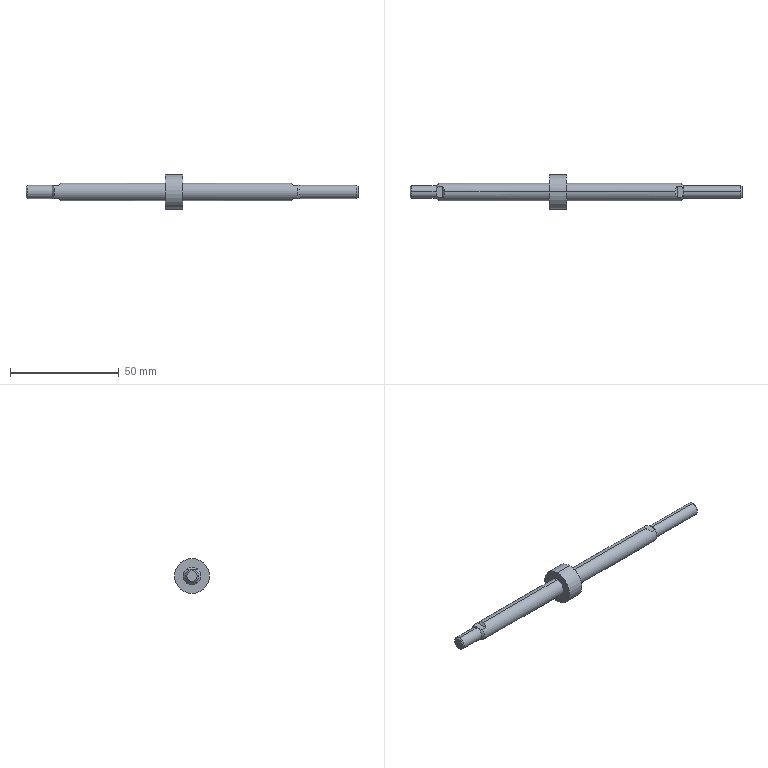Part | STEP file | _ACQJ-16x40-B10_r(40-10) | 1 solid | 30 faces | box 152.5 x 16 x 16 mm | volume 7956 mm3 | plane 12 | cylinder 10 | cone 8 | commonest cylinder face diameters 6 x4 8 x4 16 x2
STEP:
#1=CARTESIAN_POINT('',(107.2,2.646,-3.));
#2=VERTEX_POINT('',#1);
#3=CARTESIAN_POINT('',(106.2,0.,-4.));
#4=VERTEX_POINT('',#3);
#5=CARTESIAN_POINT('',(107.2,2.646,-3.));
#6=CARTESIAN_POINT('',(106.548,1.907,-3.652));
#7=CARTESIAN_POINT('',(106.2,0.9852,-4.));
#8=CARTESIAN_POINT('',(106.2,0.,-4.));
#9=(BOUNDED_CURVE()B_SPLINE_CURVE(3,(#5,#6,#7,#8),.UNSPECIFIED.,.F.,.F.)B_SPLINE_CURVE_WITH_KNOTS((4,4),(5.56,6.283),.UNSPECIFIED.)CURVE()GEOMETRIC_REPRESENTATION_ITEM()RATIONAL_B_SPLINE_CURVE((1.,0.9569,0.9569,1.))REPRESENTATION_ITEM(''));
#10=EDGE_CURVE('',#2,#4,#9,.T.);
#11=ORIENTED_EDGE('',*,*,#10,.T.);
#12=CARTESIAN_POINT('',(56.55,0.,-4.));
#13=VERTEX_POINT('',#12);
#14=CARTESIAN_POINT('',(137.,0.,-4.));
#15=DIRECTION('',(-1.,0.,0.));
#16=VECTOR('',#15,1000.);
#17=LINE('',#14,#16);
#18=EDGE_CURVE('',#4,#13,#17,.T.);
#19=ORIENTED_EDGE('',*,*,#18,.T.);
#20=CARTESIAN_POINT('',(56.55,0.,4.));
#21=VERTEX_POINT('',#20);
#22=CARTESIAN_POINT('',(56.55,0.,0.));
#23=DIRECTION('',(1.,0.,0.));
#24=DIRECTION('',(0.,0.,1.));
#25=AXIS2_PLACEMENT_3D('',#22,#23,#24);
#26=CIRCLE('',#25,4.);
#27=EDGE_CURVE('',#13,#21,#26,.T.);
#28=ORIENTED_EDGE('',*,*,#27,.T.);
#29=CARTESIAN_POINT('',(106.2,0.,4.));
#30=VERTEX_POINT('',#29);
#31=CARTESIAN_POINT('',(137.,0.,4.));
#32=DIRECTION('',(-1.,0.,0.));
#33=VECTOR('',#32,1000.);
#34=LINE('',#31,#33);
#35=EDGE_CURVE('',#30,#21,#34,.T.);
#36=ORIENTED_EDGE('',*,*,#35,.F.);
#37=CARTESIAN_POINT('',(107.2,2.646,3.));
#38=VERTEX_POINT('',#37);
#39=CARTESIAN_POINT('',(106.2,0.,4.));
#40=CARTESIAN_POINT('',(106.2,0.9852,4.));
#41=CARTESIAN_POINT('',(106.548,1.907,3.652));
#42=CARTESIAN_POINT('',(107.2,2.646,3.));
#43=(BOUNDED_CURVE()B_SPLINE_CURVE(3,(#39,#40,#41,#42),.UNSPECIFIED.,.F.,.F.)B_SPLINE_CURVE_WITH_KNOTS((4,4),(0.,0.7227),.UNSPECIFIED.)CURVE()GEOMETRIC_REPRESENTATION_ITEM()RATIONAL_B_SPLINE_CURVE((1.,0.9569,0.9569,1.))REPRESENTATION_ITEM(''));
#44=EDGE_CURVE('',#30,#38,#43,.T.);
#45=ORIENTED_EDGE('',*,*,#44,.T.);
#46=CARTESIAN_POINT('',(109.2,2.646,3.));
#47=VERTEX_POINT('',#46);
#48=CARTESIAN_POINT('',(137.,2.646,3.));
#49=DIRECTION('',(1.,0.,0.));
#50=VECTOR('',#49,1000.);
#51=LINE('',#48,#50);
#52=EDGE_CURVE('',#38,#47,#51,.T.);
#53=ORIENTED_EDGE('',*,*,#52,.T.);
#54=CARTESIAN_POINT('',(109.2,2.646,-3.));
#55=VERTEX_POINT('',#54);
#56=CARTESIAN_POINT('',(109.2,0.,0.));
#57=DIRECTION('',(-1.,0.,0.));
#58=DIRECTION('',(0.,0.,1.));
#59=AXIS2_PLACEMENT_3D('',#56,#57,#58);
#60=CIRCLE('',#59,4.);
#61=EDGE_CURVE('',#47,#55,#60,.T.);
#62=ORIENTED_EDGE('',*,*,#61,.T.);
#63=CARTESIAN_POINT('',(137.,2.646,-3.));
#64=DIRECTION('',(-1.,0.,0.));
#65=VECTOR('',#64,1000.);
#66=LINE('',#63,#65);
#67=EDGE_CURVE('',#55,#2,#66,.T.);
#68=ORIENTED_EDGE('',*,*,#67,.T.);
#69=EDGE_LOOP('',(#11,#19,#28,#36,#45,#53,#62,#68));
#70=FACE_OUTER_BOUND('',#69,.T.);
#71=CARTESIAN_POINT('',(137.,0.,0.));
#72=DIRECTION('',(-1.,0.,0.));
#73=DIRECTION('',(0.,0.,1.));
#74=AXIS2_PLACEMENT_3D('',#71,#72,#73);
#75=CYLINDRICAL_SURFACE('',#74,4.);
#76=ADVANCED_FACE('',(#70),#75,.T.);
#77=CARTESIAN_POINT('',(56.55,0.,8.));
#78=VERTEX_POINT('',#77);
#79=CARTESIAN_POINT('',(56.55,0.,-8.));
#80=VERTEX_POINT('',#79);
#81=CARTESIAN_POINT('',(56.55,0.,0.));
#82=DIRECTION('',(-1.,0.,0.));
#83=DIRECTION('',(0.,0.,1.));
#84=AXIS2_PLACEMENT_3D('',#81,#82,#83);
#85=CIRCLE('',#84,8.);
#86=EDGE_CURVE('',#78,#80,#85,.T.);
#87=ORIENTED_EDGE('',*,*,#86,.T.);
#88=CARTESIAN_POINT('',(48.5,0.,-8.));
#89=VERTEX_POINT('',#88);
#90=CARTESIAN_POINT('',(56.55,0.,-8.));
#91=DIRECTION('',(-1.,0.,0.));
#92=VECTOR('',#91,1000.);
#93=LINE('',#90,#92);
#94=EDGE_CURVE('',#80,#89,#93,.T.);
#95=ORIENTED_EDGE('',*,*,#94,.T.);
#96=CARTESIAN_POINT('',(48.5,0.,8.));
#97=VERTEX_POINT('',#96);
#98=CARTESIAN_POINT('',(48.5,0.,0.));
#99=DIRECTION('',(1.,0.,0.));
#100=DIRECTION('',(0.,0.,1.));
#101=AXIS2_PLACEMENT_3D('',#98,#99,#100);
#102=CIRCLE('',#101,8.);
#103=EDGE_CURVE('',#89,#97,#102,.T.);
#104=ORIENTED_EDGE('',*,*,#103,.T.);
#105=CARTESIAN_POINT('',(56.55,0.,8.));
#106=DIRECTION('',(-1.,0.,0.));
#107=VECTOR('',#106,1000.);
#108=LINE('',#105,#107);
#109=EDGE_CURVE('',#78,#97,#108,.T.);
#110=ORIENTED_EDGE('',*,*,#109,.F.);
#111=EDGE_LOOP('',(#87,#95,#104,#110));
#112=FACE_OUTER_BOUND('',#111,.T.);
#113=CARTESIAN_POINT('',(56.55,0.,0.));
#114=DIRECTION('',(-1.,0.,0.));
#115=DIRECTION('',(0.,0.,1.));
#116=AXIS2_PLACEMENT_3D('',#113,#114,#115);
#117=CYLINDRICAL_SURFACE('',#116,8.);
#118=ADVANCED_FACE('',(#112),#117,.T.);
#119=CARTESIAN_POINT('',(136.387,0.,3.));
#120=VERTEX_POINT('',#119);
#121=CARTESIAN_POINT('',(136.387,0.,-3.));
#122=VERTEX_POINT('',#121);
#123=CARTESIAN_POINT('',(136.387,0.,0.));
#124=DIRECTION('',(-1.,0.,0.));
#125=DIRECTION('',(0.,0.,1.));
#126=AXIS2_PLACEMENT_3D('',#123,#124,#125);
#127=CIRCLE('',#126,3.);
#128=EDGE_CURVE('',#120,#122,#127,.T.);
#129=ORIENTED_EDGE('',*,*,#128,.T.);
#130=CARTESIAN_POINT('',(110.2,0.,-3.));
#131=VERTEX_POINT('',#130);
#132=CARTESIAN_POINT('',(137.,0.,-3.));
#133=DIRECTION('',(-1.,0.,0.));
#134=VECTOR('',#133,1000.);
#135=LINE('',#132,#134);
#136=EDGE_CURVE('',#122,#131,#135,.T.);
#137=ORIENTED_EDGE('',*,*,#136,.T.);
#138=CARTESIAN_POINT('',(110.2,0.,3.));
#139=VERTEX_POINT('',#138);
#140=CARTESIAN_POINT('',(110.2,0.,0.));
#141=DIRECTION('',(-1.,0.,0.));
#142=DIRECTION('',(0.,0.,1.));
#143=AXIS2_PLACEMENT_3D('',#140,#141,#142);
#144=CIRCLE('',#143,3.);
#145=EDGE_CURVE('',#139,#131,#144,.T.);
#146=ORIENTED_EDGE('',*,*,#145,.F.);
#147=CARTESIAN_POINT('',(137.,0.,3.));
#148=DIRECTION('',(-1.,0.,0.));
#149=VECTOR('',#148,1000.);
#150=LINE('',#147,#149);
#151=EDGE_CURVE('',#120,#139,#150,.T.);
#152=ORIENTED_EDGE('',*,*,#151,.F.);
#153=EDGE_LOOP('',(#129,#137,#146,#152));
#154=FACE_OUTER_BOUND('',#153,.T.);
#155=CARTESIAN_POINT('',(137.,0.,0.));
#156=DIRECTION('',(-1.,0.,0.));
#157=DIRECTION('',(0.,0.,1.));
#158=AXIS2_PLACEMENT_3D('',#155,#156,#157);
#159=CYLINDRICAL_SURFACE('',#158,3.);
#160=ADVANCED_FACE('',(#154),#159,.T.);
#161=CARTESIAN_POINT('',(137.,0.,2.386));
#162=VERTEX_POINT('',#161);
#163=CARTESIAN_POINT('',(137.,0.,-2.386));
#164=VERTEX_POINT('',#163);
#165=CARTESIAN_POINT('',(137.,0.,0.));
#166=DIRECTION('',(-1.,0.,0.));
#167=DIRECTION('',(0.,0.,1.));
#168=AXIS2_PLACEMENT_3D('',#165,#166,#167);
#169=CIRCLE('',#168,2.386);
#170=EDGE_CURVE('',#162,#164,#169,.T.);
#171=ORIENTED_EDGE('',*,*,#170,.T.);
#172=CARTESIAN_POINT('',(136.387,0.,-3.));
#173=DIRECTION('',(-0.7071,0.,-0.7071));
#174=VECTOR('',#173,1000.);
#175=LINE('',#172,#174);
#176=EDGE_CURVE('',#164,#122,#175,.T.);
#177=ORIENTED_EDGE('',*,*,#176,.T.);
#178=ORIENTED_EDGE('',*,*,#128,.F.);
#179=CARTESIAN_POINT('',(136.387,0.,3.));
#180=DIRECTION('',(-0.7071,0.,0.7071));
#181=VECTOR('',#180,1000.);
#182=LINE('',#179,#181);
#183=EDGE_CURVE('',#162,#120,#182,.T.);
#184=ORIENTED_EDGE('',*,*,#183,.F.);
#185=EDGE_LOOP('',(#171,#177,#178,#184));
#186=FACE_OUTER_BOUND('',#185,.T.);
#187=CARTESIAN_POINT('',(136.387,0.,0.));
#188=DIRECTION('',(-1.,0.,0.));
#189=DIRECTION('',(0.,0.,1.));
#190=AXIS2_PLACEMENT_3D('',#187,#188,#189);
#191=CONICAL_SURFACE('',#190,3.,0.7854);
#192=ADVANCED_FACE('',(#186),#191,.T.);
#193=CARTESIAN_POINT('',(48.5,0.,4.));
#194=VERTEX_POINT('',#193);
#195=CARTESIAN_POINT('',(48.5,0.,-4.));
#196=VERTEX_POINT('',#195);
#197=CARTESIAN_POINT('',(48.5,0.,0.));
#198=DIRECTION('',(-1.,0.,0.));
#199=DIRECTION('',(0.,0.,1.));
#200=AXIS2_PLACEMENT_3D('',#197,#198,#199);
#201=CIRCLE('',#200,4.);
#202=EDGE_CURVE('',#194,#196,#201,.T.);
#203=ORIENTED_EDGE('',*,*,#202,.T.);
#204=CARTESIAN_POINT('',(0.5,0.,-4.));
#205=VERTEX_POINT('',#204);
#206=CARTESIAN_POINT('',(56.55,0.,-4.));
#207=DIRECTION('',(-1.,0.,0.));
#208=VECTOR('',#207,1000.);
#209=LINE('',#206,#208);
#210=EDGE_CURVE('',#196,#205,#209,.T.);
#211=ORIENTED_EDGE('',*,*,#210,.T.);
#212=CARTESIAN_POINT('',(-0.5,2.646,-3.));
#213=VERTEX_POINT('',#212);
#214=CARTESIAN_POINT('',(0.5,0.,-4.));
#215=CARTESIAN_POINT('',(0.5,0.9852,-4.));
#216=CARTESIAN_POINT('',(0.1517,1.907,-3.652));
#217=CARTESIAN_POINT('',(-0.5,2.646,-3.));
#218=(BOUNDED_CURVE()B_SPLINE_CURVE(3,(#214,#215,#216,#217),.UNSPECIFIED.,.F.,.F.)B_SPLINE_CURVE_WITH_KNOTS((4,4),(3.142,3.864),.UNSPECIFIED.)CURVE()GEOMETRIC_REPRESENTATION_ITEM()RATIONAL_B_SPLINE_CURVE((1.,0.9569,0.9569,1.))REPRESENTATION_ITEM(''));
#219=EDGE_CURVE('',#205,#213,#218,.T.);
#220=ORIENTED_EDGE('',*,*,#219,.T.);
#221=CARTESIAN_POINT('',(-2.5,2.646,-3.));
#222=VERTEX_POINT('',#221);
#223=CARTESIAN_POINT('',(56.55,2.646,-3.));
#224=DIRECTION('',(-1.,0.,0.));
#225=VECTOR('',#224,1000.);
#226=LINE('',#223,#225);
#227=EDGE_CURVE('',#213,#222,#226,.T.);
#228=ORIENTED_EDGE('',*,*,#227,.T.);
#229=CARTESIAN_POINT('',(-2.5,2.646,3.));
#230=VERTEX_POINT('',#229);
#231=CARTESIAN_POINT('',(-2.5,0.,0.));
#232=DIRECTION('',(1.,0.,0.));
#233=DIRECTION('',(0.,0.,1.));
#234=AXIS2_PLACEMENT_3D('',#231,#232,#233);
#235=CIRCLE('',#234,4.);
#236=EDGE_CURVE('',#222,#230,#235,.T.);
#237=ORIENTED_EDGE('',*,*,#236,.T.);
#238=CARTESIAN_POINT('',(-0.5,2.646,3.));
#239=VERTEX_POINT('',#238);
#240=CARTESIAN_POINT('',(56.55,2.646,3.));
#241=DIRECTION('',(1.,0.,0.));
#242=VECTOR('',#241,1000.);
#243=LINE('',#240,#242);
#244=EDGE_CURVE('',#230,#239,#243,.T.);
#245=ORIENTED_EDGE('',*,*,#244,.T.);
#246=CARTESIAN_POINT('',(0.5,0.,4.));
#247=VERTEX_POINT('',#246);
#248=CARTESIAN_POINT('',(-0.5,2.646,3.));
#249=CARTESIAN_POINT('',(0.1517,1.907,3.652));
#250=CARTESIAN_POINT('',(0.5,0.9852,4.));
#251=CARTESIAN_POINT('',(0.5,0.,4.));
#252=(BOUNDED_CURVE()B_SPLINE_CURVE(3,(#248,#249,#250,#251),.UNSPECIFIED.,.F.,.T.)B_SPLINE_CURVE_WITH_KNOTS((4,4),(2.419,3.142),.UNSPECIFIED.)CURVE()GEOMETRIC_REPRESENTATION_ITEM()RATIONAL_B_SPLINE_CURVE((1.,0.9569,0.9569,1.))REPRESENTATION_ITEM(''));
#253=EDGE_CURVE('',#239,#247,#252,.T.);
#254=ORIENTED_EDGE('',*,*,#253,.T.);
#255=CARTESIAN_POINT('',(56.55,0.,4.));
#256=DIRECTION('',(-1.,0.,0.));
#257=VECTOR('',#256,1000.);
#258=LINE('',#255,#257);
#259=EDGE_CURVE('',#194,#247,#258,.T.);
#260=ORIENTED_EDGE('',*,*,#259,.F.);
#261=EDGE_LOOP('',(#203,#211,#220,#228,#237,#245,#254,#260));
#262=FACE_OUTER_BOUND('',#261,.T.);
#263=CARTESIAN_POINT('',(56.55,0.,0.));
#264=DIRECTION('',(-1.,0.,0.));
#265=DIRECTION('',(0.,0.,1.));
#266=AXIS2_PLACEMENT_3D('',#263,#264,#265);
#267=CYLINDRICAL_SURFACE('',#266,4.);
#268=ADVANCED_FACE('',(#262),#267,.T.);
#269=CARTESIAN_POINT('',(-3.5,0.,-3.));
#270=VERTEX_POINT('',#269);
#271=CARTESIAN_POINT('',(-3.5,0.,3.));
#272=VERTEX_POINT('',#271);
#273=CARTESIAN_POINT('',(-3.5,0.,0.));
#274=DIRECTION('',(1.,0.,0.));
#275=DIRECTION('',(0.,0.,-1.));
#276=AXIS2_PLACEMENT_3D('',#273,#274,#275);
#277=CIRCLE('',#276,3.);
#278=EDGE_CURVE('',#270,#272,#277,.T.);
#279=ORIENTED_EDGE('',*,*,#278,.F.);
#280=CARTESIAN_POINT('',(-14.886,0.,-3.));
#281=VERTEX_POINT('',#280);
#282=CARTESIAN_POINT('',(0.,0.,-3.));
#283=DIRECTION('',(-1.,0.,0.));
#284=VECTOR('',#283,1000.);
#285=LINE('',#282,#284);
#286=EDGE_CURVE('',#270,#281,#285,.T.);
#287=ORIENTED_EDGE('',*,*,#286,.T.);
#288=CARTESIAN_POINT('',(-14.886,0.,3.));
#289=VERTEX_POINT('',#288);
#290=CARTESIAN_POINT('',(-14.886,0.,0.));
#291=DIRECTION('',(1.,0.,0.));
#292=DIRECTION('',(0.,0.,1.));
#293=AXIS2_PLACEMENT_3D('',#290,#291,#292);
#294=CIRCLE('',#293,3.);
#295=EDGE_CURVE('',#281,#289,#294,.T.);
#296=ORIENTED_EDGE('',*,*,#295,.T.);
#297=CARTESIAN_POINT('',(0.,0.,3.));
#298=DIRECTION('',(-1.,0.,0.));
#299=VECTOR('',#298,1000.);
#300=LINE('',#297,#299);
#301=EDGE_CURVE('',#272,#289,#300,.T.);
#302=ORIENTED_EDGE('',*,*,#301,.F.);
#303=EDGE_LOOP('',(#279,#287,#296,#302));
#304=FACE_OUTER_BOUND('',#303,.T.);
#305=CARTESIAN_POINT('',(0.,0.,0.));
#306=DIRECTION('',(-1.,0.,0.));
#307=DIRECTION('',(0.,0.,1.));
#308=AXIS2_PLACEMENT_3D('',#305,#306,#307);
#309=CYLINDRICAL_SURFACE('',#308,3.);
#310=ADVANCED_FACE('',(#304),#309,.T.);
#311=CARTESIAN_POINT('',(-15.5,0.,-2.387));
#312=VERTEX_POINT('',#311);
#313=CARTESIAN_POINT('',(-15.5,0.,2.387));
#314=VERTEX_POINT('',#313);
#315=CARTESIAN_POINT('',(-15.5,0.,0.));
#316=DIRECTION('',(1.,0.,0.));
#317=DIRECTION('',(0.,0.,-1.));
#318=AXIS2_PLACEMENT_3D('',#315,#316,#317);
#319=CIRCLE('',#318,2.387);
#320=EDGE_CURVE('',#312,#314,#319,.T.);
#321=ORIENTED_EDGE('',*,*,#320,.T.);
#322=CARTESIAN_POINT('',(-14.887,0.,3.));
#323=DIRECTION('',(0.7071,0.,0.7071));
#324=VECTOR('',#323,1000.);
#325=LINE('',#322,#324);
#326=EDGE_CURVE('',#314,#289,#325,.T.);
#327=ORIENTED_EDGE('',*,*,#326,.T.);
#328=ORIENTED_EDGE('',*,*,#295,.F.);
#329=CARTESIAN_POINT('',(-14.887,0.,-3.));
#330=DIRECTION('',(0.7071,0.,-0.7071));
#331=VECTOR('',#330,1000.);
#332=LINE('',#329,#331);
#333=EDGE_CURVE('',#312,#281,#332,.T.);
#334=ORIENTED_EDGE('',*,*,#333,.F.);
#335=EDGE_LOOP('',(#321,#327,#328,#334));
#336=FACE_OUTER_BOUND('',#335,.T.);
#337=CARTESIAN_POINT('',(-14.887,0.,0.));
#338=DIRECTION('',(1.,0.,0.));
#339=DIRECTION('',(0.,0.,-1.));
#340=AXIS2_PLACEMENT_3D('',#337,#338,#339);
#341=CONICAL_SURFACE('',#340,3.,0.7854);
#342=ADVANCED_FACE('',(#336),#341,.T.);
#343=ORIENTED_EDGE('',*,*,#18,.F.);
#344=CARTESIAN_POINT('',(107.2,-2.646,-3.));
#345=VERTEX_POINT('',#344);
#346=CARTESIAN_POINT('',(106.2,0.,-4.));
#347=CARTESIAN_POINT('',(106.2,-0.9852,-4.));
#348=CARTESIAN_POINT('',(106.548,-1.907,-3.652));
#349=CARTESIAN_POINT('',(107.2,-2.646,-3.));
#350=(BOUNDED_CURVE()B_SPLINE_CURVE(3,(#346,#347,#348,#349),.UNSPECIFIED.,.F.,.T.)B_SPLINE_CURVE_WITH_KNOTS((4,4),(0.,0.7227),.UNSPECIFIED.)CURVE()GEOMETRIC_REPRESENTATION_ITEM()RATIONAL_B_SPLINE_CURVE((1.,0.9569,0.9569,1.))REPRESENTATION_ITEM(''));
#351=EDGE_CURVE('',#4,#345,#350,.T.);
#352=ORIENTED_EDGE('',*,*,#351,.T.);
#353=CARTESIAN_POINT('',(109.2,-2.646,-3.));
#354=VERTEX_POINT('',#353);
#355=CARTESIAN_POINT('',(137.,-2.646,-3.));
#356=DIRECTION('',(1.,0.,0.));
#357=VECTOR('',#356,1000.);
#358=LINE('',#355,#357);
#359=EDGE_CURVE('',#345,#354,#358,.T.);
#360=ORIENTED_EDGE('',*,*,#359,.T.);
#361=CARTESIAN_POINT('',(109.2,-2.646,3.));
#362=VERTEX_POINT('',#361);
#363=CARTESIAN_POINT('',(109.2,0.,0.));
#364=DIRECTION('',(-1.,0.,0.));
#365=DIRECTION('',(0.,0.,1.));
#366=AXIS2_PLACEMENT_3D('',#363,#364,#365);
#367=CIRCLE('',#366,4.);
#368=EDGE_CURVE('',#354,#362,#367,.T.);
#369=ORIENTED_EDGE('',*,*,#368,.T.);
#370=CARTESIAN_POINT('',(107.2,-2.646,3.));
#371=VERTEX_POINT('',#370);
#372=CARTESIAN_POINT('',(137.,-2.646,3.));
#373=DIRECTION('',(-1.,0.,0.));
#374=VECTOR('',#373,1000.);
#375=LINE('',#372,#374);
#376=EDGE_CURVE('',#362,#371,#375,.T.);
#377=ORIENTED_EDGE('',*,*,#376,.T.);
#378=CARTESIAN_POINT('',(107.2,-2.646,3.));
#379=CARTESIAN_POINT('',(106.548,-1.907,3.652));
#380=CARTESIAN_POINT('',(106.2,-0.9852,4.));
#381=CARTESIAN_POINT('',(106.2,0.,4.));
#382=(BOUNDED_CURVE()B_SPLINE_CURVE(3,(#378,#379,#380,#381),.UNSPECIFIED.,.F.,.F.)B_SPLINE_CURVE_WITH_KNOTS((4,4),(5.56,6.283),.UNSPECIFIED.)CURVE()GEOMETRIC_REPRESENTATION_ITEM()RATIONAL_B_SPLINE_CURVE((1.,0.9569,0.9569,1.))REPRESENTATION_ITEM(''));
#383=EDGE_CURVE('',#371,#30,#382,.T.);
#384=ORIENTED_EDGE('',*,*,#383,.T.);
#385=ORIENTED_EDGE('',*,*,#35,.T.);
#386=CARTESIAN_POINT('',(56.55,0.,0.));
#387=DIRECTION('',(1.,0.,0.));
#388=DIRECTION('',(0.,0.,1.));
#389=AXIS2_PLACEMENT_3D('',#386,#387,#388);
#390=CIRCLE('',#389,4.);
#391=EDGE_CURVE('',#21,#13,#390,.T.);
#392=ORIENTED_EDGE('',*,*,#391,.T.);
#393=EDGE_LOOP('',(#343,#352,#360,#369,#377,#384,#385,#392));
#394=FACE_OUTER_BOUND('',#393,.T.);
#395=CARTESIAN_POINT('',(137.,0.,0.));
#396=DIRECTION('',(-1.,0.,0.));
#397=DIRECTION('',(0.,0.,1.));
#398=AXIS2_PLACEMENT_3D('',#395,#396,#397);
#399=CYLINDRICAL_SURFACE('',#398,4.);
#400=ADVANCED_FACE('',(#394),#399,.T.);
#401=ORIENTED_EDGE('',*,*,#86,.F.);
#402=CARTESIAN_POINT('',(56.55,0.,0.));
#403=DIRECTION('',(-1.,0.,0.));
#404=DIRECTION('',(0.,0.,1.));
#405=AXIS2_PLACEMENT_3D('',#402,#403,#404);
#406=CIRCLE('',#405,8.);
#407=EDGE_CURVE('',#80,#78,#406,.T.);
#408=ORIENTED_EDGE('',*,*,#407,.F.);
#409=EDGE_LOOP('',(#401,#408));
#410=FACE_OUTER_BOUND('',#409,.T.);
#411=ORIENTED_EDGE('',*,*,#391,.F.);
#412=ORIENTED_EDGE('',*,*,#27,.F.);
#413=EDGE_LOOP('',(#411,#412));
#414=FACE_BOUND('',#413,.T.);
#415=CARTESIAN_POINT('',(56.55,8.,0.));
#416=DIRECTION('',(-1.,0.,0.));
#417=DIRECTION('',(0.,0.,1.));
#418=AXIS2_PLACEMENT_3D('',#415,#416,#417);
#419=PLANE('',#418);
#420=ADVANCED_FACE('',(#410,#414),#419,.F.);
#421=ORIENTED_EDGE('',*,*,#52,.F.);
#422=CARTESIAN_POINT('',(107.2,6.,3.));
#423=DIRECTION('',(0.,-1.,0.));
#424=VECTOR('',#423,1000.);
#425=LINE('',#422,#424);
#426=EDGE_CURVE('',#38,#371,#425,.T.);
#427=ORIENTED_EDGE('',*,*,#426,.T.);
#428=ORIENTED_EDGE('',*,*,#376,.F.);
#429=CARTESIAN_POINT('',(109.2,-2.646,3.));
#430=CARTESIAN_POINT('',(109.464,-2.246,3.));
#431=CARTESIAN_POINT('',(109.706,-1.835,3.));
#432=CARTESIAN_POINT('',(109.984,-1.176,3.));
#433=CARTESIAN_POINT('',(110.063,-0.946,3.));
#434=CARTESIAN_POINT('',(110.17,-0.4792,3.));
#435=CARTESIAN_POINT('',(110.2,-0.2419,3.));
#436=CARTESIAN_POINT('',(110.2,0.,3.));
#437=B_SPLINE_CURVE_WITH_KNOTS('',3,(#429,#430,#431,#432,#433,#434,#435,#436),.UNSPECIFIED.,.F.,.F.,(4,2,2,4),(0.,0.001428,0.002142,0.002856),.UNSPECIFIED.);
#438=EDGE_CURVE('',#362,#139,#437,.T.);
#439=ORIENTED_EDGE('',*,*,#438,.T.);
#440=CARTESIAN_POINT('',(110.2,0.,3.));
#441=CARTESIAN_POINT('',(110.2,0.2419,3.));
#442=CARTESIAN_POINT('',(110.17,0.4786,3.));
#443=CARTESIAN_POINT('',(110.063,0.9437,3.));
#444=CARTESIAN_POINT('',(109.985,1.173,3.));
#445=CARTESIAN_POINT('',(109.706,1.834,3.));
#446=CARTESIAN_POINT('',(109.464,2.246,3.));
#447=CARTESIAN_POINT('',(109.2,2.646,3.));
#448=B_SPLINE_CURVE_WITH_KNOTS('',3,(#440,#441,#442,#443,#444,#445,#446,#447),.UNSPECIFIED.,.F.,.F.,(4,2,2,4),(0.,0.0007149,0.00143,0.00286),.UNSPECIFIED.);
#449=EDGE_CURVE('',#139,#47,#448,.T.);
#450=ORIENTED_EDGE('',*,*,#449,.T.);
#451=EDGE_LOOP('',(#421,#427,#428,#439,#450));
#452=FACE_OUTER_BOUND('',#451,.T.);
#453=CARTESIAN_POINT('',(110.2,6.,3.));
#454=DIRECTION('',(0.,0.,1.));
#455=DIRECTION('',(1.,0.,0.));
#456=AXIS2_PLACEMENT_3D('',#453,#454,#455);
#457=PLANE('',#456);
#458=ADVANCED_FACE('',(#452),#457,.T.);
#459=ORIENTED_EDGE('',*,*,#383,.F.);
#460=ORIENTED_EDGE('',*,*,#426,.F.);
#461=ORIENTED_EDGE('',*,*,#44,.F.);
#462=EDGE_LOOP('',(#459,#460,#461));
#463=FACE_OUTER_BOUND('',#462,.T.);
#464=CARTESIAN_POINT('',(107.2,6.,3.));
#465=DIRECTION('',(0.7071,0.,0.7071));
#466=DIRECTION('',(0.7071,0.,-0.7071));
#467=AXIS2_PLACEMENT_3D('',#464,#465,#466);
#468=PLANE('',#467);
#469=ADVANCED_FACE('',(#463),#468,.T.);
#470=ORIENTED_EDGE('',*,*,#438,.F.);
#471=ORIENTED_EDGE('',*,*,#368,.F.);
#472=CARTESIAN_POINT('',(109.2,-2.646,-3.));
#473=CARTESIAN_POINT('',(109.464,-2.246,-3.));
#474=CARTESIAN_POINT('',(109.706,-1.835,-3.));
#475=CARTESIAN_POINT('',(109.984,-1.176,-3.));
#476=CARTESIAN_POINT('',(110.063,-0.946,-3.));
#477=CARTESIAN_POINT('',(110.17,-0.4792,-3.));
#478=CARTESIAN_POINT('',(110.2,-0.2419,-3.));
#479=CARTESIAN_POINT('',(110.2,0.,-3.));
#480=B_SPLINE_CURVE_WITH_KNOTS('',3,(#472,#473,#474,#475,#476,#477,#478,#479),.UNSPECIFIED.,.F.,.F.,(4,2,2,4),(0.,0.001428,0.002142,0.002856),.UNSPECIFIED.);
#481=EDGE_CURVE('',#354,#131,#480,.T.);
#482=ORIENTED_EDGE('',*,*,#481,.T.);
#483=CARTESIAN_POINT('',(110.2,0.,0.));
#484=DIRECTION('',(-1.,0.,0.));
#485=DIRECTION('',(0.,0.,1.));
#486=AXIS2_PLACEMENT_3D('',#483,#484,#485);
#487=CIRCLE('',#486,3.);
#488=EDGE_CURVE('',#131,#139,#487,.T.);
#489=ORIENTED_EDGE('',*,*,#488,.T.);
#490=EDGE_LOOP('',(#470,#471,#482,#489));
#491=FACE_OUTER_BOUND('',#490,.T.);
#492=CARTESIAN_POINT('',(109.2,0.,0.));
#493=DIRECTION('',(-1.,0.,0.));
#494=DIRECTION('',(0.,0.,1.));
#495=AXIS2_PLACEMENT_3D('',#492,#493,#494);
#496=CONICAL_SURFACE('',#495,4.,0.7854);
#497=ADVANCED_FACE('',(#491),#496,.T.);
#498=ORIENTED_EDGE('',*,*,#359,.F.);
#499=CARTESIAN_POINT('',(107.2,6.,-3.));
#500=DIRECTION('',(0.,1.,0.));
#501=VECTOR('',#500,1000.);
#502=LINE('',#499,#501);
#503=EDGE_CURVE('',#345,#2,#502,.T.);
#504=ORIENTED_EDGE('',*,*,#503,.T.);
#505=ORIENTED_EDGE('',*,*,#67,.F.);
#506=CARTESIAN_POINT('',(109.2,2.646,-3.));
#507=CARTESIAN_POINT('',(109.464,2.246,-3.));
#508=CARTESIAN_POINT('',(109.706,1.835,-3.));
#509=CARTESIAN_POINT('',(109.984,1.176,-3.));
#510=CARTESIAN_POINT('',(110.063,0.946,-3.));
#511=CARTESIAN_POINT('',(110.17,0.4792,-3.));
#512=CARTESIAN_POINT('',(110.2,0.2419,-3.));
#513=CARTESIAN_POINT('',(110.2,0.,-3.));
#514=B_SPLINE_CURVE_WITH_KNOTS('',3,(#506,#507,#508,#509,#510,#511,#512,#513),.UNSPECIFIED.,.F.,.F.,(4,2,2,4),(0.,0.001428,0.002142,0.002856),.UNSPECIFIED.);
#515=EDGE_CURVE('',#55,#131,#514,.T.);
#516=ORIENTED_EDGE('',*,*,#515,.T.);
#517=ORIENTED_EDGE('',*,*,#481,.F.);
#518=EDGE_LOOP('',(#498,#504,#505,#516,#517));
#519=FACE_OUTER_BOUND('',#518,.T.);
#520=CARTESIAN_POINT('',(107.2,6.,-3.));
#521=DIRECTION('',(0.,0.,-1.));
#522=DIRECTION('',(-1.,0.,0.));
#523=AXIS2_PLACEMENT_3D('',#520,#521,#522);
#524=PLANE('',#523);
#525=ADVANCED_FACE('',(#519),#524,.T.);
#526=ORIENTED_EDGE('',*,*,#10,.F.);
#527=ORIENTED_EDGE('',*,*,#503,.F.);
#528=ORIENTED_EDGE('',*,*,#351,.F.);
#529=EDGE_LOOP('',(#526,#527,#528));
#530=FACE_OUTER_BOUND('',#529,.T.);
#531=CARTESIAN_POINT('',(100.129,6.,-10.071));
#532=DIRECTION('',(0.7071,0.,-0.7071));
#533=DIRECTION('',(-0.7071,0.,-0.7071));
#534=AXIS2_PLACEMENT_3D('',#531,#532,#533);
#535=PLANE('',#534);
#536=ADVANCED_FACE('',(#530),#535,.T.);
#537=ORIENTED_EDGE('',*,*,#515,.F.);
#538=ORIENTED_EDGE('',*,*,#61,.F.);
#539=ORIENTED_EDGE('',*,*,#449,.F.);
#540=ORIENTED_EDGE('',*,*,#145,.T.);
#541=EDGE_LOOP('',(#537,#538,#539,#540));
#542=FACE_OUTER_BOUND('',#541,.T.);
#543=CARTESIAN_POINT('',(109.2,0.,0.));
#544=DIRECTION('',(-1.,0.,0.));
#545=DIRECTION('',(0.,0.,1.));
#546=AXIS2_PLACEMENT_3D('',#543,#544,#545);
#547=CONICAL_SURFACE('',#546,4.,0.7854);
#548=ADVANCED_FACE('',(#542),#547,.T.);
#549=ORIENTED_EDGE('',*,*,#94,.F.);
#550=ORIENTED_EDGE('',*,*,#407,.T.);
#551=ORIENTED_EDGE('',*,*,#109,.T.);
#552=CARTESIAN_POINT('',(48.5,0.,0.));
#553=DIRECTION('',(1.,0.,0.));
#554=DIRECTION('',(0.,0.,1.));
#555=AXIS2_PLACEMENT_3D('',#552,#553,#554);
#556=CIRCLE('',#555,8.);
#557=EDGE_CURVE('',#97,#89,#556,.T.);
#558=ORIENTED_EDGE('',*,*,#557,.T.);
#559=EDGE_LOOP('',(#549,#550,#551,#558));
#560=FACE_OUTER_BOUND('',#559,.T.);
#561=CARTESIAN_POINT('',(56.55,0.,0.));
#562=DIRECTION('',(-1.,0.,0.));
#563=DIRECTION('',(0.,0.,1.));
#564=AXIS2_PLACEMENT_3D('',#561,#562,#563);
#565=CYLINDRICAL_SURFACE('',#564,8.);
#566=ADVANCED_FACE('',(#560),#565,.T.);
#567=ORIENTED_EDGE('',*,*,#136,.F.);
#568=CARTESIAN_POINT('',(136.387,0.,0.));
#569=DIRECTION('',(-1.,0.,0.));
#570=DIRECTION('',(0.,0.,1.));
#571=AXIS2_PLACEMENT_3D('',#568,#569,#570);
#572=CIRCLE('',#571,3.);
#573=EDGE_CURVE('',#122,#120,#572,.T.);
#574=ORIENTED_EDGE('',*,*,#573,.T.);
#575=ORIENTED_EDGE('',*,*,#151,.T.);
#576=ORIENTED_EDGE('',*,*,#488,.F.);
#577=EDGE_LOOP('',(#567,#574,#575,#576));
#578=FACE_OUTER_BOUND('',#577,.T.);
#579=CARTESIAN_POINT('',(137.,0.,0.));
#580=DIRECTION('',(-1.,0.,0.));
#581=DIRECTION('',(0.,0.,1.));
#582=AXIS2_PLACEMENT_3D('',#579,#580,#581);
#583=CYLINDRICAL_SURFACE('',#582,3.);
#584=ADVANCED_FACE('',(#578),#583,.T.);
#585=ORIENTED_EDGE('',*,*,#202,.F.);
#586=CARTESIAN_POINT('',(48.5,0.,0.));
#587=DIRECTION('',(-1.,0.,0.));
#588=DIRECTION('',(0.,0.,1.));
#589=AXIS2_PLACEMENT_3D('',#586,#587,#588);
#590=CIRCLE('',#589,4.);
#591=EDGE_CURVE('',#196,#194,#590,.T.);
#592=ORIENTED_EDGE('',*,*,#591,.F.);
#593=EDGE_LOOP('',(#585,#592));
#594=FACE_BOUND('',#593,.T.);
#595=ORIENTED_EDGE('',*,*,#557,.F.);
#596=ORIENTED_EDGE('',*,*,#103,.F.);
#597=EDGE_LOOP('',(#595,#596));
#598=FACE_OUTER_BOUND('',#597,.T.);
#599=CARTESIAN_POINT('',(48.5,4.,0.));
#600=DIRECTION('',(1.,0.,0.));
#601=DIRECTION('',(0.,0.,-1.));
#602=AXIS2_PLACEMENT_3D('',#599,#600,#601);
#603=PLANE('',#602);
#604=ADVANCED_FACE('',(#594,#598),#603,.F.);
#605=ORIENTED_EDGE('',*,*,#176,.F.);
#606=CARTESIAN_POINT('',(137.,0.,0.));
#607=DIRECTION('',(-1.,0.,0.));
#608=DIRECTION('',(0.,0.,1.));
#609=AXIS2_PLACEMENT_3D('',#606,#607,#608);
#610=CIRCLE('',#609,2.386);
#611=EDGE_CURVE('',#164,#162,#610,.T.);
#612=ORIENTED_EDGE('',*,*,#611,.T.);
#613=ORIENTED_EDGE('',*,*,#183,.T.);
#614=ORIENTED_EDGE('',*,*,#573,.F.);
#615=EDGE_LOOP('',(#605,#612,#613,#614));
#616=FACE_OUTER_BOUND('',#615,.T.);
#617=CARTESIAN_POINT('',(136.387,0.,0.));
#618=DIRECTION('',(-1.,0.,0.));
#619=DIRECTION('',(0.,0.,1.));
#620=AXIS2_PLACEMENT_3D('',#617,#618,#619);
#621=CONICAL_SURFACE('',#620,3.,0.7854);
#622=ADVANCED_FACE('',(#616),#621,.T.);
#623=ORIENTED_EDGE('',*,*,#210,.F.);
#624=ORIENTED_EDGE('',*,*,#591,.T.);
#625=ORIENTED_EDGE('',*,*,#259,.T.);
#626=CARTESIAN_POINT('',(-0.5,-2.646,3.));
#627=VERTEX_POINT('',#626);
#628=CARTESIAN_POINT('',(0.5,0.,4.));
#629=CARTESIAN_POINT('',(0.5,-0.9852,4.));
#630=CARTESIAN_POINT('',(0.1517,-1.907,3.652));
#631=CARTESIAN_POINT('',(-0.5,-2.646,3.));
#632=(BOUNDED_CURVE()B_SPLINE_CURVE(3,(#628,#629,#630,#631),.UNSPECIFIED.,.F.,.F.)B_SPLINE_CURVE_WITH_KNOTS((4,4),(3.142,3.864),.UNSPECIFIED.)CURVE()GEOMETRIC_REPRESENTATION_ITEM()RATIONAL_B_SPLINE_CURVE((1.,0.9569,0.9569,1.))REPRESENTATION_ITEM(''));
#633=EDGE_CURVE('',#247,#627,#632,.T.);
#634=ORIENTED_EDGE('',*,*,#633,.T.);
#635=CARTESIAN_POINT('',(-2.5,-2.646,3.));
#636=VERTEX_POINT('',#635);
#637=CARTESIAN_POINT('',(56.55,-2.646,3.));
#638=DIRECTION('',(-1.,0.,0.));
#639=VECTOR('',#638,1000.);
#640=LINE('',#637,#639);
#641=EDGE_CURVE('',#627,#636,#640,.T.);
#642=ORIENTED_EDGE('',*,*,#641,.T.);
#643=CARTESIAN_POINT('',(-2.5,-2.646,-3.));
#644=VERTEX_POINT('',#643);
#645=CARTESIAN_POINT('',(-2.5,0.,0.));
#646=DIRECTION('',(1.,0.,0.));
#647=DIRECTION('',(0.,0.,1.));
#648=AXIS2_PLACEMENT_3D('',#645,#646,#647);
#649=CIRCLE('',#648,4.);
#650=EDGE_CURVE('',#636,#644,#649,.T.);
#651=ORIENTED_EDGE('',*,*,#650,.T.);
#652=CARTESIAN_POINT('',(-0.5,-2.646,-3.));
#653=VERTEX_POINT('',#652);
#654=CARTESIAN_POINT('',(56.55,-2.646,-3.));
#655=DIRECTION('',(1.,0.,0.));
#656=VECTOR('',#655,1000.);
#657=LINE('',#654,#656);
#658=EDGE_CURVE('',#644,#653,#657,.T.);
#659=ORIENTED_EDGE('',*,*,#658,.T.);
#660=CARTESIAN_POINT('',(-0.5,-2.646,-3.));
#661=CARTESIAN_POINT('',(0.1517,-1.907,-3.652));
#662=CARTESIAN_POINT('',(0.5,-0.9852,-4.));
#663=CARTESIAN_POINT('',(0.5,0.,-4.));
#664=(BOUNDED_CURVE()B_SPLINE_CURVE(3,(#660,#661,#662,#663),.UNSPECIFIED.,.F.,.F.)B_SPLINE_CURVE_WITH_KNOTS((4,4),(2.419,3.142),.UNSPECIFIED.)CURVE()GEOMETRIC_REPRESENTATION_ITEM()RATIONAL_B_SPLINE_CURVE((1.,0.9569,0.9569,1.))REPRESENTATION_ITEM(''));
#665=EDGE_CURVE('',#653,#205,#664,.T.);
#666=ORIENTED_EDGE('',*,*,#665,.T.);
#667=EDGE_LOOP('',(#623,#624,#625,#634,#642,#651,#659,#666));
#668=FACE_OUTER_BOUND('',#667,.T.);
#669=CARTESIAN_POINT('',(56.55,0.,0.));
#670=DIRECTION('',(-1.,0.,0.));
#671=DIRECTION('',(0.,0.,1.));
#672=AXIS2_PLACEMENT_3D('',#669,#670,#671);
#673=CYLINDRICAL_SURFACE('',#672,4.);
#674=ADVANCED_FACE('',(#668),#673,.T.);
#675=ORIENTED_EDGE('',*,*,#170,.F.);
#676=ORIENTED_EDGE('',*,*,#611,.F.);
#677=EDGE_LOOP('',(#675,#676));
#678=FACE_OUTER_BOUND('',#677,.T.);
#679=CARTESIAN_POINT('',(137.,2.386,0.));
#680=DIRECTION('',(-1.,0.,0.));
#681=DIRECTION('',(0.,0.,1.));
#682=AXIS2_PLACEMENT_3D('',#679,#680,#681);
#683=PLANE('',#682);
#684=ADVANCED_FACE('',(#678),#683,.F.);
#685=ORIENTED_EDGE('',*,*,#253,.F.);
#686=CARTESIAN_POINT('',(-0.5,6.,3.));
#687=DIRECTION('',(0.,-1.,0.));
#688=VECTOR('',#687,1000.);
#689=LINE('',#686,#688);
#690=EDGE_CURVE('',#239,#627,#689,.T.);
#691=ORIENTED_EDGE('',*,*,#690,.T.);
#692=ORIENTED_EDGE('',*,*,#633,.F.);
#693=EDGE_LOOP('',(#685,#691,#692));
#694=FACE_OUTER_BOUND('',#693,.T.);
#695=CARTESIAN_POINT('',(19.5,6.,23.));
#696=DIRECTION('',(-0.7071,0.,0.7071));
#697=DIRECTION('',(0.7071,0.,0.7071));
#698=AXIS2_PLACEMENT_3D('',#695,#696,#697);
#699=PLANE('',#698);
#700=ADVANCED_FACE('',(#694),#699,.T.);
#701=CARTESIAN_POINT('',(-2.5,2.646,3.));
#702=CARTESIAN_POINT('',(-2.764,2.246,3.));
#703=CARTESIAN_POINT('',(-3.006,1.835,3.));
#704=CARTESIAN_POINT('',(-3.284,1.176,3.));
#705=CARTESIAN_POINT('',(-3.363,0.946,3.));
#706=CARTESIAN_POINT('',(-3.47,0.4792,3.));
#707=CARTESIAN_POINT('',(-3.5,0.2419,3.));
#708=CARTESIAN_POINT('',(-3.5,0.,3.));
#709=B_SPLINE_CURVE_WITH_KNOTS('',3,(#701,#702,#703,#704,#705,#706,#707,#708),.UNSPECIFIED.,.F.,.F.,(4,2,2,4),(0.,0.001428,0.002142,0.002856),.UNSPECIFIED.);
#710=EDGE_CURVE('',#230,#272,#709,.T.);
#711=ORIENTED_EDGE('',*,*,#710,.T.);
#712=CARTESIAN_POINT('',(-3.5,0.,3.));
#713=CARTESIAN_POINT('',(-3.5,-0.2419,3.));
#714=CARTESIAN_POINT('',(-3.47,-0.4786,3.));
#715=CARTESIAN_POINT('',(-3.363,-0.9437,3.));
#716=CARTESIAN_POINT('',(-3.285,-1.173,3.));
#717=CARTESIAN_POINT('',(-3.006,-1.834,3.));
#718=CARTESIAN_POINT('',(-2.764,-2.246,3.));
#719=CARTESIAN_POINT('',(-2.5,-2.646,3.));
#720=B_SPLINE_CURVE_WITH_KNOTS('',3,(#712,#713,#714,#715,#716,#717,#718,#719),.UNSPECIFIED.,.F.,.F.,(4,2,2,4),(0.,0.0007149,0.00143,0.00286),.UNSPECIFIED.);
#721=EDGE_CURVE('',#272,#636,#720,.T.);
#722=ORIENTED_EDGE('',*,*,#721,.T.);
#723=ORIENTED_EDGE('',*,*,#641,.F.);
#724=ORIENTED_EDGE('',*,*,#690,.F.);
#725=ORIENTED_EDGE('',*,*,#244,.F.);
#726=EDGE_LOOP('',(#711,#722,#723,#724,#725));
#727=FACE_OUTER_BOUND('',#726,.T.);
#728=CARTESIAN_POINT('',(-0.5,6.,3.));
#729=DIRECTION('',(0.,0.,1.));
#730=DIRECTION('',(1.,0.,0.));
#731=AXIS2_PLACEMENT_3D('',#728,#729,#730);
#732=PLANE('',#731);
#733=ADVANCED_FACE('',(#727),#732,.T.);
#734=ORIENTED_EDGE('',*,*,#710,.F.);
#735=ORIENTED_EDGE('',*,*,#236,.F.);
#736=CARTESIAN_POINT('',(-2.5,2.646,-3.));
#737=CARTESIAN_POINT('',(-2.764,2.246,-3.));
#738=CARTESIAN_POINT('',(-3.006,1.835,-3.));
#739=CARTESIAN_POINT('',(-3.284,1.176,-3.));
#740=CARTESIAN_POINT('',(-3.363,0.946,-3.));
#741=CARTESIAN_POINT('',(-3.47,0.4792,-3.));
#742=CARTESIAN_POINT('',(-3.5,0.2419,-3.));
#743=CARTESIAN_POINT('',(-3.5,0.,-3.));
#744=B_SPLINE_CURVE_WITH_KNOTS('',3,(#736,#737,#738,#739,#740,#741,#742,#743),.UNSPECIFIED.,.F.,.F.,(4,2,2,4),(0.,0.001428,0.002142,0.002856),.UNSPECIFIED.);
#745=EDGE_CURVE('',#222,#270,#744,.T.);
#746=ORIENTED_EDGE('',*,*,#745,.T.);
#747=ORIENTED_EDGE('',*,*,#278,.T.);
#748=EDGE_LOOP('',(#734,#735,#746,#747));
#749=FACE_OUTER_BOUND('',#748,.T.);
#750=CARTESIAN_POINT('',(-2.5,0.,0.));
#751=DIRECTION('',(1.,0.,0.));
#752=DIRECTION('',(0.,0.,-1.));
#753=AXIS2_PLACEMENT_3D('',#750,#751,#752);
#754=CONICAL_SURFACE('',#753,4.,0.7854);
#755=ADVANCED_FACE('',(#749),#754,.T.);
#756=CARTESIAN_POINT('',(-2.5,-2.646,-3.));
#757=CARTESIAN_POINT('',(-2.764,-2.246,-3.));
#758=CARTESIAN_POINT('',(-3.006,-1.835,-3.));
#759=CARTESIAN_POINT('',(-3.284,-1.176,-3.));
#760=CARTESIAN_POINT('',(-3.363,-0.946,-3.));
#761=CARTESIAN_POINT('',(-3.47,-0.4792,-3.));
#762=CARTESIAN_POINT('',(-3.5,-0.2419,-3.));
#763=CARTESIAN_POINT('',(-3.5,0.,-3.));
#764=B_SPLINE_CURVE_WITH_KNOTS('',3,(#756,#757,#758,#759,#760,#761,#762,#763),.UNSPECIFIED.,.F.,.F.,(4,2,2,4),(0.,0.001428,0.002142,0.002856),.UNSPECIFIED.);
#765=EDGE_CURVE('',#644,#270,#764,.T.);
#766=ORIENTED_EDGE('',*,*,#765,.T.);
#767=ORIENTED_EDGE('',*,*,#745,.F.);
#768=ORIENTED_EDGE('',*,*,#227,.F.);
#769=CARTESIAN_POINT('',(-0.5,6.,-3.));
#770=DIRECTION('',(0.,-1.,0.));
#771=VECTOR('',#770,1000.);
#772=LINE('',#769,#771);
#773=EDGE_CURVE('',#213,#653,#772,.T.);
#774=ORIENTED_EDGE('',*,*,#773,.T.);
#775=ORIENTED_EDGE('',*,*,#658,.F.);
#776=EDGE_LOOP('',(#766,#767,#768,#774,#775));
#777=FACE_OUTER_BOUND('',#776,.T.);
#778=CARTESIAN_POINT('',(-3.5,6.,-3.));
#779=DIRECTION('',(0.,0.,-1.));
#780=DIRECTION('',(-1.,0.,0.));
#781=AXIS2_PLACEMENT_3D('',#778,#779,#780);
#782=PLANE('',#781);
#783=ADVANCED_FACE('',(#777),#782,.T.);
#784=ORIENTED_EDGE('',*,*,#665,.F.);
#785=ORIENTED_EDGE('',*,*,#773,.F.);
#786=ORIENTED_EDGE('',*,*,#219,.F.);
#787=EDGE_LOOP('',(#784,#785,#786));
#788=FACE_OUTER_BOUND('',#787,.T.);
#789=CARTESIAN_POINT('',(-0.5,6.,-3.));
#790=DIRECTION('',(-0.7071,0.,-0.7071));
#791=DIRECTION('',(-0.7071,0.,0.7071));
#792=AXIS2_PLACEMENT_3D('',#789,#790,#791);
#793=PLANE('',#792);
#794=ADVANCED_FACE('',(#788),#793,.T.);
#795=ORIENTED_EDGE('',*,*,#765,.F.);
#796=ORIENTED_EDGE('',*,*,#650,.F.);
#797=ORIENTED_EDGE('',*,*,#721,.F.);
#798=CARTESIAN_POINT('',(-3.5,0.,0.));
#799=DIRECTION('',(1.,0.,0.));
#800=DIRECTION('',(0.,0.,-1.));
#801=AXIS2_PLACEMENT_3D('',#798,#799,#800);
#802=CIRCLE('',#801,3.);
#803=EDGE_CURVE('',#272,#270,#802,.T.);
#804=ORIENTED_EDGE('',*,*,#803,.T.);
#805=EDGE_LOOP('',(#795,#796,#797,#804));
#806=FACE_OUTER_BOUND('',#805,.T.);
#807=CARTESIAN_POINT('',(-2.5,0.,0.));
#808=DIRECTION('',(1.,0.,0.));
#809=DIRECTION('',(0.,0.,-1.));
#810=AXIS2_PLACEMENT_3D('',#807,#808,#809);
#811=CONICAL_SURFACE('',#810,4.,0.7854);
#812=ADVANCED_FACE('',(#806),#811,.T.);
#813=ORIENTED_EDGE('',*,*,#286,.F.);
#814=ORIENTED_EDGE('',*,*,#803,.F.);
#815=ORIENTED_EDGE('',*,*,#301,.T.);
#816=CARTESIAN_POINT('',(-14.886,0.,0.));
#817=DIRECTION('',(1.,0.,0.));
#818=DIRECTION('',(0.,0.,1.));
#819=AXIS2_PLACEMENT_3D('',#816,#817,#818);
#820=CIRCLE('',#819,3.);
#821=EDGE_CURVE('',#289,#281,#820,.T.);
#822=ORIENTED_EDGE('',*,*,#821,.T.);
#823=EDGE_LOOP('',(#813,#814,#815,#822));
#824=FACE_OUTER_BOUND('',#823,.T.);
#825=CARTESIAN_POINT('',(0.,0.,0.));
#826=DIRECTION('',(-1.,0.,0.));
#827=DIRECTION('',(0.,0.,1.));
#828=AXIS2_PLACEMENT_3D('',#825,#826,#827);
#829=CYLINDRICAL_SURFACE('',#828,3.);
#830=ADVANCED_FACE('',(#824),#829,.T.);
#831=ORIENTED_EDGE('',*,*,#326,.F.);
#832=CARTESIAN_POINT('',(-15.5,0.,0.));
#833=DIRECTION('',(1.,0.,0.));
#834=DIRECTION('',(0.,0.,-1.));
#835=AXIS2_PLACEMENT_3D('',#832,#833,#834);
#836=CIRCLE('',#835,2.387);
#837=EDGE_CURVE('',#314,#312,#836,.T.);
#838=ORIENTED_EDGE('',*,*,#837,.T.);
#839=ORIENTED_EDGE('',*,*,#333,.T.);
#840=ORIENTED_EDGE('',*,*,#821,.F.);
#841=EDGE_LOOP('',(#831,#838,#839,#840));
#842=FACE_OUTER_BOUND('',#841,.T.);
#843=CARTESIAN_POINT('',(-14.887,0.,0.));
#844=DIRECTION('',(1.,0.,0.));
#845=DIRECTION('',(0.,0.,-1.));
#846=AXIS2_PLACEMENT_3D('',#843,#844,#845);
#847=CONICAL_SURFACE('',#846,3.,0.7854);
#848=ADVANCED_FACE('',(#842),#847,.T.);
#849=ORIENTED_EDGE('',*,*,#320,.F.);
#850=ORIENTED_EDGE('',*,*,#837,.F.);
#851=EDGE_LOOP('',(#849,#850));
#852=FACE_OUTER_BOUND('',#851,.T.);
#853=CARTESIAN_POINT('',(-15.5,0.,0.));
#854=DIRECTION('',(1.,0.,0.));
#855=DIRECTION('',(0.,0.,-1.));
#856=AXIS2_PLACEMENT_3D('',#853,#854,#855);
#857=PLANE('',#856);
#858=ADVANCED_FACE('',(#852),#857,.F.);
#859=CLOSED_SHELL('',(#76,#118,#160,#192,#268,#310,#342,#400,#420,#458,#469,#497,#525,#536,#548,#566,#584,#604,#622,#674,#684,#700,#733,#755,#783,#794,#812,#830,#848,#858));
#860=MANIFOLD_SOLID_BREP('',#859);
#861=CARTESIAN_POINT('',(0.,0.,0.));
#862=DIRECTION('',(0.,0.,1.));
#863=DIRECTION('',(1.,0.,0.));
#864=AXIS2_PLACEMENT_3D('',#861,#862,#863);
#865=(LENGTH_UNIT()NAMED_UNIT(*)SI_UNIT(.MILLI.,.METRE.));
#866=UNCERTAINTY_MEASURE_WITH_UNIT(LENGTH_MEASURE(0.00001),#865,'','');
#867=(NAMED_UNIT(*)PLANE_ANGLE_UNIT()SI_UNIT($,.RADIAN.));
#868=(NAMED_UNIT(*)SI_UNIT($,.STERADIAN.)SOLID_ANGLE_UNIT());
#869=(GEOMETRIC_REPRESENTATION_CONTEXT(3)GLOBAL_UNCERTAINTY_ASSIGNED_CONTEXT((#866))GLOBAL_UNIT_ASSIGNED_CONTEXT((#865,#867,#868))REPRESENTATION_CONTEXT('',''));
#870=ADVANCED_BREP_SHAPE_REPRESENTATION('',(#860,#864),#869);